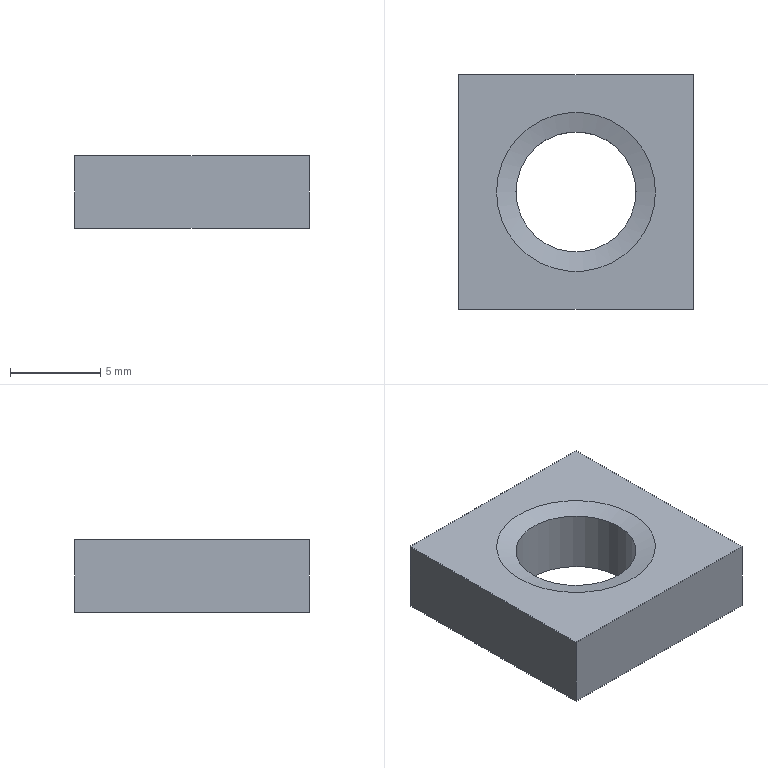Part | STEP file | Left | 1 solid | 9 faces | box 13 x 13 x 4 mm | volume 530.018 mm3 | plane 6 | cone 2 | cylinder 1 | commonest cylinder face diameters 6.647 x1
STEP:
#1=CARTESIAN_POINT('',(0.,0.,0.));
#2=DIRECTION('',(0.,0.,1.));
#3=DIRECTION('',(1.,0.,0.));
#4=AXIS2_PLACEMENT_3D('',#1,#2,#3);
#5=CARTESIAN_POINT('',(-6.5,-6.5,0.));
#6=VERTEX_POINT('',#5);
#7=CARTESIAN_POINT('',(-6.5,-6.5,4.));
#8=VERTEX_POINT('',#7);
#9=CARTESIAN_POINT('',(-6.5,-6.5,0.));
#10=DIRECTION('',(0.,0.,1.));
#11=VECTOR('',#10,1.);
#12=LINE('',#9,#11);
#13=CARTESIAN_POINT('',(-6.5,-6.5,0.));
#14=DIRECTION('',(1.,0.,0.));
#15=DIRECTION('',(0.,0.,1.));
#16=AXIS2_PLACEMENT_3D('',#13,#14,#15);
#17=PLANE('',#16);
#18=CARTESIAN_POINT('',(0.,0.));
#19=DIRECTION('',(1.,0.));
#20=VECTOR('',#19,1.);
#21=LINE('',#18,#20);
#22=(GEOMETRIC_REPRESENTATION_CONTEXT(2)PARAMETRIC_REPRESENTATION_CONTEXT()REPRESENTATION_CONTEXT('',''));
#23=DEFINITIONAL_REPRESENTATION('',(#21),#22);
#24=PCURVE('',#17,#23);
#25=CARTESIAN_POINT('',(-6.5,-6.5,0.));
#26=DIRECTION('',(0.,1.,0.));
#27=DIRECTION('',(0.,0.,1.));
#28=AXIS2_PLACEMENT_3D('',#25,#26,#27);
#29=PLANE('',#28);
#30=CARTESIAN_POINT('',(0.,0.));
#31=DIRECTION('',(1.,0.));
#32=VECTOR('',#31,1.);
#33=LINE('',#30,#32);
#34=(GEOMETRIC_REPRESENTATION_CONTEXT(2)PARAMETRIC_REPRESENTATION_CONTEXT()REPRESENTATION_CONTEXT('',''));
#35=DEFINITIONAL_REPRESENTATION('',(#33),#34);
#36=PCURVE('',#29,#35);
#37=SURFACE_CURVE('',#12,(#24,#36),.PCURVE_S1.);
#38=EDGE_CURVE('',#6,#8,#37,.T.);
#39=ORIENTED_EDGE('',*,*,#38,.F.);
#40=CARTESIAN_POINT('',(-6.5,6.5,0.));
#41=VERTEX_POINT('',#40);
#42=CARTESIAN_POINT('',(-6.5,-6.5,0.));
#43=DIRECTION('',(0.,1.,0.));
#44=VECTOR('',#43,1.);
#45=LINE('',#42,#44);
#46=CARTESIAN_POINT('',(0.,0.));
#47=DIRECTION('',(0.,-1.));
#48=VECTOR('',#47,1.);
#49=LINE('',#46,#48);
#50=(GEOMETRIC_REPRESENTATION_CONTEXT(2)PARAMETRIC_REPRESENTATION_CONTEXT()REPRESENTATION_CONTEXT('',''));
#51=DEFINITIONAL_REPRESENTATION('',(#49),#50);
#52=PCURVE('',#17,#51);
#53=CARTESIAN_POINT('',(-6.5,-6.5,0.));
#54=DIRECTION('',(0.,0.,1.));
#55=DIRECTION('',(1.,0.,0.));
#56=AXIS2_PLACEMENT_3D('',#53,#54,#55);
#57=PLANE('',#56);
#58=CARTESIAN_POINT('',(0.,0.));
#59=DIRECTION('',(0.,1.));
#60=VECTOR('',#59,1.);
#61=LINE('',#58,#60);
#62=(GEOMETRIC_REPRESENTATION_CONTEXT(2)PARAMETRIC_REPRESENTATION_CONTEXT()REPRESENTATION_CONTEXT('',''));
#63=DEFINITIONAL_REPRESENTATION('',(#61),#62);
#64=PCURVE('',#57,#63);
#65=SURFACE_CURVE('',#45,(#52,#64),.PCURVE_S1.);
#66=EDGE_CURVE('',#6,#41,#65,.T.);
#67=ORIENTED_EDGE('',*,*,#66,.T.);
#68=CARTESIAN_POINT('',(-6.5,6.5,4.));
#69=VERTEX_POINT('',#68);
#70=CARTESIAN_POINT('',(-6.5,6.5,0.));
#71=DIRECTION('',(0.,0.,1.));
#72=VECTOR('',#71,1.);
#73=LINE('',#70,#72);
#74=CARTESIAN_POINT('',(0.,-13.));
#75=DIRECTION('',(1.,0.));
#76=VECTOR('',#75,1.);
#77=LINE('',#74,#76);
#78=(GEOMETRIC_REPRESENTATION_CONTEXT(2)PARAMETRIC_REPRESENTATION_CONTEXT()REPRESENTATION_CONTEXT('',''));
#79=DEFINITIONAL_REPRESENTATION('',(#77),#78);
#80=PCURVE('',#17,#79);
#81=CARTESIAN_POINT('',(-6.5,6.5,0.));
#82=DIRECTION('',(0.,1.,0.));
#83=DIRECTION('',(0.,0.,1.));
#84=AXIS2_PLACEMENT_3D('',#81,#82,#83);
#85=PLANE('',#84);
#86=CARTESIAN_POINT('',(0.,0.));
#87=DIRECTION('',(1.,0.));
#88=VECTOR('',#87,1.);
#89=LINE('',#86,#88);
#90=(GEOMETRIC_REPRESENTATION_CONTEXT(2)PARAMETRIC_REPRESENTATION_CONTEXT()REPRESENTATION_CONTEXT('',''));
#91=DEFINITIONAL_REPRESENTATION('',(#89),#90);
#92=PCURVE('',#85,#91);
#93=SURFACE_CURVE('',#73,(#80,#92),.PCURVE_S1.);
#94=EDGE_CURVE('',#41,#69,#93,.T.);
#95=ORIENTED_EDGE('',*,*,#94,.T.);
#96=CARTESIAN_POINT('',(-6.5,-6.5,4.));
#97=DIRECTION('',(0.,1.,0.));
#98=VECTOR('',#97,1.);
#99=LINE('',#96,#98);
#100=CARTESIAN_POINT('',(4.,0.));
#101=DIRECTION('',(0.,-1.));
#102=VECTOR('',#101,1.);
#103=LINE('',#100,#102);
#104=(GEOMETRIC_REPRESENTATION_CONTEXT(2)PARAMETRIC_REPRESENTATION_CONTEXT()REPRESENTATION_CONTEXT('',''));
#105=DEFINITIONAL_REPRESENTATION('',(#103),#104);
#106=PCURVE('',#17,#105);
#107=CARTESIAN_POINT('',(-6.5,-6.5,4.));
#108=DIRECTION('',(0.,0.,1.));
#109=DIRECTION('',(1.,0.,0.));
#110=AXIS2_PLACEMENT_3D('',#107,#108,#109);
#111=PLANE('',#110);
#112=CARTESIAN_POINT('',(0.,0.));
#113=DIRECTION('',(0.,1.));
#114=VECTOR('',#113,1.);
#115=LINE('',#112,#114);
#116=(GEOMETRIC_REPRESENTATION_CONTEXT(2)PARAMETRIC_REPRESENTATION_CONTEXT()REPRESENTATION_CONTEXT('',''));
#117=DEFINITIONAL_REPRESENTATION('',(#115),#116);
#118=PCURVE('',#111,#117);
#119=SURFACE_CURVE('',#99,(#106,#118),.PCURVE_S1.);
#120=EDGE_CURVE('',#8,#69,#119,.T.);
#121=ORIENTED_EDGE('',*,*,#120,.F.);
#122=EDGE_LOOP('',(#39,#67,#95,#121));
#123=FACE_BOUND('',#122,.F.);
#124=ADVANCED_FACE('',(#123),#17,.F.);
#125=CARTESIAN_POINT('',(6.5,-6.5,0.));
#126=VERTEX_POINT('',#125);
#127=CARTESIAN_POINT('',(-6.5,-6.5,0.));
#128=DIRECTION('',(1.,0.,0.));
#129=VECTOR('',#128,1.);
#130=LINE('',#127,#129);
#131=CARTESIAN_POINT('',(0.,0.));
#132=DIRECTION('',(0.,1.));
#133=VECTOR('',#132,1.);
#134=LINE('',#131,#133);
#135=(GEOMETRIC_REPRESENTATION_CONTEXT(2)PARAMETRIC_REPRESENTATION_CONTEXT()REPRESENTATION_CONTEXT('',''));
#136=DEFINITIONAL_REPRESENTATION('',(#134),#135);
#137=PCURVE('',#29,#136);
#138=CARTESIAN_POINT('',(0.,0.));
#139=DIRECTION('',(1.,0.));
#140=VECTOR('',#139,1.);
#141=LINE('',#138,#140);
#142=(GEOMETRIC_REPRESENTATION_CONTEXT(2)PARAMETRIC_REPRESENTATION_CONTEXT()REPRESENTATION_CONTEXT('',''));
#143=DEFINITIONAL_REPRESENTATION('',(#141),#142);
#144=PCURVE('',#57,#143);
#145=SURFACE_CURVE('',#130,(#137,#144),.PCURVE_S1.);
#146=EDGE_CURVE('',#6,#126,#145,.T.);
#147=ORIENTED_EDGE('',*,*,#146,.F.);
#148=ORIENTED_EDGE('',*,*,#38,.T.);
#149=CARTESIAN_POINT('',(6.5,-6.5,4.));
#150=VERTEX_POINT('',#149);
#151=CARTESIAN_POINT('',(-6.5,-6.5,4.));
#152=DIRECTION('',(1.,0.,0.));
#153=VECTOR('',#152,1.);
#154=LINE('',#151,#153);
#155=CARTESIAN_POINT('',(4.,0.));
#156=DIRECTION('',(0.,1.));
#157=VECTOR('',#156,1.);
#158=LINE('',#155,#157);
#159=(GEOMETRIC_REPRESENTATION_CONTEXT(2)PARAMETRIC_REPRESENTATION_CONTEXT()REPRESENTATION_CONTEXT('',''));
#160=DEFINITIONAL_REPRESENTATION('',(#158),#159);
#161=PCURVE('',#29,#160);
#162=CARTESIAN_POINT('',(0.,0.));
#163=DIRECTION('',(1.,0.));
#164=VECTOR('',#163,1.);
#165=LINE('',#162,#164);
#166=(GEOMETRIC_REPRESENTATION_CONTEXT(2)PARAMETRIC_REPRESENTATION_CONTEXT()REPRESENTATION_CONTEXT('',''));
#167=DEFINITIONAL_REPRESENTATION('',(#165),#166);
#168=PCURVE('',#111,#167);
#169=SURFACE_CURVE('',#154,(#161,#168),.PCURVE_S1.);
#170=EDGE_CURVE('',#8,#150,#169,.T.);
#171=ORIENTED_EDGE('',*,*,#170,.T.);
#172=CARTESIAN_POINT('',(6.5,-6.5,0.));
#173=DIRECTION('',(0.,0.,1.));
#174=VECTOR('',#173,1.);
#175=LINE('',#172,#174);
#176=CARTESIAN_POINT('',(0.,13.));
#177=DIRECTION('',(1.,0.));
#178=VECTOR('',#177,1.);
#179=LINE('',#176,#178);
#180=(GEOMETRIC_REPRESENTATION_CONTEXT(2)PARAMETRIC_REPRESENTATION_CONTEXT()REPRESENTATION_CONTEXT('',''));
#181=DEFINITIONAL_REPRESENTATION('',(#179),#180);
#182=PCURVE('',#29,#181);
#183=CARTESIAN_POINT('',(6.5,-6.5,0.));
#184=DIRECTION('',(1.,0.,0.));
#185=DIRECTION('',(0.,0.,1.));
#186=AXIS2_PLACEMENT_3D('',#183,#184,#185);
#187=PLANE('',#186);
#188=CARTESIAN_POINT('',(0.,0.));
#189=DIRECTION('',(1.,0.));
#190=VECTOR('',#189,1.);
#191=LINE('',#188,#190);
#192=(GEOMETRIC_REPRESENTATION_CONTEXT(2)PARAMETRIC_REPRESENTATION_CONTEXT()REPRESENTATION_CONTEXT('',''));
#193=DEFINITIONAL_REPRESENTATION('',(#191),#192);
#194=PCURVE('',#187,#193);
#195=SURFACE_CURVE('',#175,(#182,#194),.PCURVE_S1.);
#196=EDGE_CURVE('',#126,#150,#195,.T.);
#197=ORIENTED_EDGE('',*,*,#196,.F.);
#198=EDGE_LOOP('',(#147,#148,#171,#197));
#199=FACE_BOUND('',#198,.F.);
#200=ADVANCED_FACE('',(#199),#29,.F.);
#201=ORIENTED_EDGE('',*,*,#120,.F.);
#202=ORIENTED_EDGE('',*,*,#170,.T.);
#203=CARTESIAN_POINT('',(6.5,6.5,4.));
#204=VERTEX_POINT('',#203);
#205=CARTESIAN_POINT('',(6.5,-6.5,4.));
#206=DIRECTION('',(0.,1.,0.));
#207=VECTOR('',#206,1.);
#208=LINE('',#205,#207);
#209=CARTESIAN_POINT('',(13.,0.));
#210=DIRECTION('',(0.,1.));
#211=VECTOR('',#210,1.);
#212=LINE('',#209,#211);
#213=(GEOMETRIC_REPRESENTATION_CONTEXT(2)PARAMETRIC_REPRESENTATION_CONTEXT()REPRESENTATION_CONTEXT('',''));
#214=DEFINITIONAL_REPRESENTATION('',(#212),#213);
#215=PCURVE('',#111,#214);
#216=CARTESIAN_POINT('',(4.,0.));
#217=DIRECTION('',(0.,-1.));
#218=VECTOR('',#217,1.);
#219=LINE('',#216,#218);
#220=(GEOMETRIC_REPRESENTATION_CONTEXT(2)PARAMETRIC_REPRESENTATION_CONTEXT()REPRESENTATION_CONTEXT('',''));
#221=DEFINITIONAL_REPRESENTATION('',(#219),#220);
#222=PCURVE('',#187,#221);
#223=SURFACE_CURVE('',#208,(#215,#222),.PCURVE_S1.);
#224=EDGE_CURVE('',#150,#204,#223,.T.);
#225=ORIENTED_EDGE('',*,*,#224,.T.);
#226=CARTESIAN_POINT('',(-6.5,6.5,4.));
#227=DIRECTION('',(1.,0.,0.));
#228=VECTOR('',#227,1.);
#229=LINE('',#226,#228);
#230=CARTESIAN_POINT('',(0.,13.));
#231=DIRECTION('',(1.,0.));
#232=VECTOR('',#231,1.);
#233=LINE('',#230,#232);
#234=(GEOMETRIC_REPRESENTATION_CONTEXT(2)PARAMETRIC_REPRESENTATION_CONTEXT()REPRESENTATION_CONTEXT('',''));
#235=DEFINITIONAL_REPRESENTATION('',(#233),#234);
#236=PCURVE('',#111,#235);
#237=CARTESIAN_POINT('',(4.,0.));
#238=DIRECTION('',(0.,1.));
#239=VECTOR('',#238,1.);
#240=LINE('',#237,#239);
#241=(GEOMETRIC_REPRESENTATION_CONTEXT(2)PARAMETRIC_REPRESENTATION_CONTEXT()REPRESENTATION_CONTEXT('',''));
#242=DEFINITIONAL_REPRESENTATION('',(#240),#241);
#243=PCURVE('',#85,#242);
#244=SURFACE_CURVE('',#229,(#236,#243),.PCURVE_S1.);
#245=EDGE_CURVE('',#69,#204,#244,.T.);
#246=ORIENTED_EDGE('',*,*,#245,.F.);
#247=EDGE_LOOP('',(#201,#202,#225,#246));
#248=FACE_BOUND('',#247,.T.);
#249=CARTESIAN_POINT('',(4.4,0.,4.));
#250=VERTEX_POINT('',#249);
#251=CARTESIAN_POINT('',(0.,0.,4.));
#252=DIRECTION('',(0.,0.,1.));
#253=DIRECTION('',(1.,0.,0.));
#254=AXIS2_PLACEMENT_3D('',#251,#252,#253);
#255=CIRCLE('',#254,4.4);
#256=CARTESIAN_POINT('',(6.5,6.5));
#257=DIRECTION('',(1.,0.));
#258=AXIS2_PLACEMENT_2D('',#256,#257);
#259=CIRCLE('',#258,4.4);
#260=(GEOMETRIC_REPRESENTATION_CONTEXT(2)PARAMETRIC_REPRESENTATION_CONTEXT()REPRESENTATION_CONTEXT('',''));
#261=DEFINITIONAL_REPRESENTATION('',(#259),#260);
#262=PCURVE('',#111,#261);
#263=CARTESIAN_POINT('',(0.,0.,3.712));
#264=DIRECTION('',(0.,0.,1.));
#265=DIRECTION('',(1.,0.,0.));
#266=AXIS2_PLACEMENT_3D('',#263,#264,#265);
#267=CONICAL_SURFACE('',#266,3.323,1.309);
#268=CARTESIAN_POINT('',(0.,0.2885));
#269=DIRECTION('',(1.,0.));
#270=VECTOR('',#269,1.);
#271=LINE('',#268,#270);
#272=(GEOMETRIC_REPRESENTATION_CONTEXT(2)PARAMETRIC_REPRESENTATION_CONTEXT()REPRESENTATION_CONTEXT('',''));
#273=DEFINITIONAL_REPRESENTATION('',(#271),#272);
#274=PCURVE('',#267,#273);
#275=SURFACE_CURVE('',#255,(#262,#274),.PCURVE_S1.);
#276=EDGE_CURVE('',#250,#250,#275,.T.);
#277=ORIENTED_EDGE('',*,*,#276,.F.);
#278=EDGE_LOOP('',(#277));
#279=FACE_BOUND('',#278,.T.);
#280=ADVANCED_FACE('',(#248,#279),#111,.T.);
#281=CARTESIAN_POINT('',(6.5,6.5,0.));
#282=VERTEX_POINT('',#281);
#283=CARTESIAN_POINT('',(-6.5,6.5,0.));
#284=DIRECTION('',(1.,0.,0.));
#285=VECTOR('',#284,1.);
#286=LINE('',#283,#285);
#287=CARTESIAN_POINT('',(0.,0.));
#288=DIRECTION('',(0.,1.));
#289=VECTOR('',#288,1.);
#290=LINE('',#287,#289);
#291=(GEOMETRIC_REPRESENTATION_CONTEXT(2)PARAMETRIC_REPRESENTATION_CONTEXT()REPRESENTATION_CONTEXT('',''));
#292=DEFINITIONAL_REPRESENTATION('',(#290),#291);
#293=PCURVE('',#85,#292);
#294=CARTESIAN_POINT('',(0.,13.));
#295=DIRECTION('',(1.,0.));
#296=VECTOR('',#295,1.);
#297=LINE('',#294,#296);
#298=(GEOMETRIC_REPRESENTATION_CONTEXT(2)PARAMETRIC_REPRESENTATION_CONTEXT()REPRESENTATION_CONTEXT('',''));
#299=DEFINITIONAL_REPRESENTATION('',(#297),#298);
#300=PCURVE('',#57,#299);
#301=SURFACE_CURVE('',#286,(#293,#300),.PCURVE_S1.);
#302=EDGE_CURVE('',#41,#282,#301,.T.);
#303=ORIENTED_EDGE('',*,*,#302,.F.);
#304=ORIENTED_EDGE('',*,*,#94,.T.);
#305=ORIENTED_EDGE('',*,*,#245,.T.);
#306=CARTESIAN_POINT('',(6.5,6.5,0.));
#307=DIRECTION('',(0.,0.,1.));
#308=VECTOR('',#307,1.);
#309=LINE('',#306,#308);
#310=CARTESIAN_POINT('',(0.,13.));
#311=DIRECTION('',(1.,0.));
#312=VECTOR('',#311,1.);
#313=LINE('',#310,#312);
#314=(GEOMETRIC_REPRESENTATION_CONTEXT(2)PARAMETRIC_REPRESENTATION_CONTEXT()REPRESENTATION_CONTEXT('',''));
#315=DEFINITIONAL_REPRESENTATION('',(#313),#314);
#316=PCURVE('',#85,#315);
#317=CARTESIAN_POINT('',(0.,-13.));
#318=DIRECTION('',(1.,0.));
#319=VECTOR('',#318,1.);
#320=LINE('',#317,#319);
#321=(GEOMETRIC_REPRESENTATION_CONTEXT(2)PARAMETRIC_REPRESENTATION_CONTEXT()REPRESENTATION_CONTEXT('',''));
#322=DEFINITIONAL_REPRESENTATION('',(#320),#321);
#323=PCURVE('',#187,#322);
#324=SURFACE_CURVE('',#309,(#316,#323),.PCURVE_S1.);
#325=EDGE_CURVE('',#282,#204,#324,.T.);
#326=ORIENTED_EDGE('',*,*,#325,.F.);
#327=EDGE_LOOP('',(#303,#304,#305,#326));
#328=FACE_BOUND('',#327,.T.);
#329=ADVANCED_FACE('',(#328),#85,.T.);
#330=ORIENTED_EDGE('',*,*,#66,.F.);
#331=ORIENTED_EDGE('',*,*,#146,.T.);
#332=CARTESIAN_POINT('',(6.5,-6.5,0.));
#333=DIRECTION('',(0.,1.,0.));
#334=VECTOR('',#333,1.);
#335=LINE('',#332,#334);
#336=CARTESIAN_POINT('',(13.,0.));
#337=DIRECTION('',(0.,1.));
#338=VECTOR('',#337,1.);
#339=LINE('',#336,#338);
#340=(GEOMETRIC_REPRESENTATION_CONTEXT(2)PARAMETRIC_REPRESENTATION_CONTEXT()REPRESENTATION_CONTEXT('',''));
#341=DEFINITIONAL_REPRESENTATION('',(#339),#340);
#342=PCURVE('',#57,#341);
#343=CARTESIAN_POINT('',(0.,0.));
#344=DIRECTION('',(0.,-1.));
#345=VECTOR('',#344,1.);
#346=LINE('',#343,#345);
#347=(GEOMETRIC_REPRESENTATION_CONTEXT(2)PARAMETRIC_REPRESENTATION_CONTEXT()REPRESENTATION_CONTEXT('',''));
#348=DEFINITIONAL_REPRESENTATION('',(#346),#347);
#349=PCURVE('',#187,#348);
#350=SURFACE_CURVE('',#335,(#342,#349),.PCURVE_S1.);
#351=EDGE_CURVE('',#126,#282,#350,.T.);
#352=ORIENTED_EDGE('',*,*,#351,.T.);
#353=ORIENTED_EDGE('',*,*,#302,.F.);
#354=EDGE_LOOP('',(#330,#331,#352,#353));
#355=FACE_BOUND('',#354,.F.);
#356=CARTESIAN_POINT('',(4.4,0.,0.));
#357=VERTEX_POINT('',#356);
#358=CARTESIAN_POINT('',(0.,0.,0.));
#359=DIRECTION('',(0.,0.,1.));
#360=DIRECTION('',(1.,0.,0.));
#361=AXIS2_PLACEMENT_3D('',#358,#359,#360);
#362=CIRCLE('',#361,4.4);
#363=CARTESIAN_POINT('',(6.5,6.5));
#364=DIRECTION('',(1.,0.));
#365=AXIS2_PLACEMENT_2D('',#363,#364);
#366=CIRCLE('',#365,4.4);
#367=(GEOMETRIC_REPRESENTATION_CONTEXT(2)PARAMETRIC_REPRESENTATION_CONTEXT()REPRESENTATION_CONTEXT('',''));
#368=DEFINITIONAL_REPRESENTATION('',(#366),#367);
#369=PCURVE('',#57,#368);
#370=CARTESIAN_POINT('',(0.,0.,0.));
#371=DIRECTION('',(0.,0.,-1.));
#372=DIRECTION('',(1.,0.,0.));
#373=AXIS2_PLACEMENT_3D('',#370,#371,#372);
#374=CONICAL_SURFACE('',#373,4.4,1.309);
#375=CARTESIAN_POINT('',(6.283,0.));
#376=DIRECTION('',(-1.,0.));
#377=VECTOR('',#376,1.);
#378=LINE('',#375,#377);
#379=(GEOMETRIC_REPRESENTATION_CONTEXT(2)PARAMETRIC_REPRESENTATION_CONTEXT()REPRESENTATION_CONTEXT('',''));
#380=DEFINITIONAL_REPRESENTATION('',(#378),#379);
#381=PCURVE('',#374,#380);
#382=SURFACE_CURVE('',#362,(#369,#381),.PCURVE_S1.);
#383=EDGE_CURVE('',#357,#357,#382,.T.);
#384=ORIENTED_EDGE('',*,*,#383,.F.);
#385=EDGE_LOOP('',(#384));
#386=FACE_BOUND('',#385,.F.);
#387=ADVANCED_FACE('',(#355,#386),#57,.F.);
#388=ORIENTED_EDGE('',*,*,#196,.F.);
#389=ORIENTED_EDGE('',*,*,#351,.T.);
#390=ORIENTED_EDGE('',*,*,#325,.T.);
#391=ORIENTED_EDGE('',*,*,#224,.F.);
#392=EDGE_LOOP('',(#388,#389,#390,#391));
#393=FACE_BOUND('',#392,.T.);
#394=ADVANCED_FACE('',(#393),#187,.T.);
#395=CARTESIAN_POINT('',(3.323,0.,3.712));
#396=VERTEX_POINT('',#395);
#397=CARTESIAN_POINT('',(3.323,0.,3.712));
#398=DIRECTION('',(0.9659,0.,0.2588));
#399=VECTOR('',#398,1.);
#400=LINE('',#397,#399);
#401=CARTESIAN_POINT('',(0.,0.));
#402=DIRECTION('',(0.,1.));
#403=VECTOR('',#402,1.);
#404=LINE('',#401,#403);
#405=(GEOMETRIC_REPRESENTATION_CONTEXT(2)PARAMETRIC_REPRESENTATION_CONTEXT()REPRESENTATION_CONTEXT('',''));
#406=DEFINITIONAL_REPRESENTATION('',(#404),#405);
#407=PCURVE('',#267,#406);
#408=CARTESIAN_POINT('',(6.283,0.));
#409=DIRECTION('',(0.,1.));
#410=VECTOR('',#409,1.);
#411=LINE('',#408,#410);
#412=(GEOMETRIC_REPRESENTATION_CONTEXT(2)PARAMETRIC_REPRESENTATION_CONTEXT()REPRESENTATION_CONTEXT('',''));
#413=DEFINITIONAL_REPRESENTATION('',(#411),#412);
#414=PCURVE('',#267,#413);
#415=SEAM_CURVE('',#400,(#407,#414),.PCURVE_S1.);
#416=EDGE_CURVE('',#396,#250,#415,.T.);
#417=ORIENTED_EDGE('',*,*,#416,.F.);
#418=CARTESIAN_POINT('',(0.,0.,3.712));
#419=DIRECTION('',(0.,0.,1.));
#420=DIRECTION('',(1.,0.,0.));
#421=AXIS2_PLACEMENT_3D('',#418,#419,#420);
#422=CIRCLE('',#421,3.323);
#423=CARTESIAN_POINT('',(0.,0.));
#424=DIRECTION('',(1.,0.));
#425=VECTOR('',#424,1.);
#426=LINE('',#423,#425);
#427=(GEOMETRIC_REPRESENTATION_CONTEXT(2)PARAMETRIC_REPRESENTATION_CONTEXT()REPRESENTATION_CONTEXT('',''));
#428=DEFINITIONAL_REPRESENTATION('',(#426),#427);
#429=PCURVE('',#267,#428);
#430=CARTESIAN_POINT('',(0.,0.,0.2885));
#431=DIRECTION('',(0.,0.,1.));
#432=DIRECTION('',(1.,0.,0.));
#433=AXIS2_PLACEMENT_3D('',#430,#431,#432);
#434=CYLINDRICAL_SURFACE('',#433,3.323);
#435=CARTESIAN_POINT('',(0.,3.423));
#436=DIRECTION('',(1.,0.));
#437=VECTOR('',#436,1.);
#438=LINE('',#435,#437);
#439=(GEOMETRIC_REPRESENTATION_CONTEXT(2)PARAMETRIC_REPRESENTATION_CONTEXT()REPRESENTATION_CONTEXT('',''));
#440=DEFINITIONAL_REPRESENTATION('',(#438),#439);
#441=PCURVE('',#434,#440);
#442=SURFACE_CURVE('',#422,(#429,#441),.PCURVE_S1.);
#443=EDGE_CURVE('',#396,#396,#442,.T.);
#444=ORIENTED_EDGE('',*,*,#443,.T.);
#445=ORIENTED_EDGE('',*,*,#416,.T.);
#446=ORIENTED_EDGE('',*,*,#276,.F.);
#447=EDGE_LOOP('',(#417,#444,#445,#446));
#448=FACE_BOUND('',#447,.F.);
#449=ADVANCED_FACE('',(#448),#267,.F.);
#450=CARTESIAN_POINT('',(3.323,0.,0.2885));
#451=VERTEX_POINT('',#450);
#452=CARTESIAN_POINT('',(4.4,0.,0.));
#453=DIRECTION('',(-0.9659,0.,0.2588));
#454=VECTOR('',#453,1.);
#455=LINE('',#452,#454);
#456=CARTESIAN_POINT('',(6.283,0.));
#457=DIRECTION('',(0.,-1.));
#458=VECTOR('',#457,1.);
#459=LINE('',#456,#458);
#460=(GEOMETRIC_REPRESENTATION_CONTEXT(2)PARAMETRIC_REPRESENTATION_CONTEXT()REPRESENTATION_CONTEXT('',''));
#461=DEFINITIONAL_REPRESENTATION('',(#459),#460);
#462=PCURVE('',#374,#461);
#463=CARTESIAN_POINT('',(0.,0.));
#464=DIRECTION('',(0.,-1.));
#465=VECTOR('',#464,1.);
#466=LINE('',#463,#465);
#467=(GEOMETRIC_REPRESENTATION_CONTEXT(2)PARAMETRIC_REPRESENTATION_CONTEXT()REPRESENTATION_CONTEXT('',''));
#468=DEFINITIONAL_REPRESENTATION('',(#466),#467);
#469=PCURVE('',#374,#468);
#470=SEAM_CURVE('',#455,(#462,#469),.PCURVE_S1.);
#471=EDGE_CURVE('',#357,#451,#470,.T.);
#472=ORIENTED_EDGE('',*,*,#471,.F.);
#473=ORIENTED_EDGE('',*,*,#383,.T.);
#474=ORIENTED_EDGE('',*,*,#471,.T.);
#475=CARTESIAN_POINT('',(0.,0.,0.2885));
#476=DIRECTION('',(0.,0.,1.));
#477=DIRECTION('',(1.,0.,0.));
#478=AXIS2_PLACEMENT_3D('',#475,#476,#477);
#479=CIRCLE('',#478,3.323);
#480=CARTESIAN_POINT('',(6.283,-0.2885));
#481=DIRECTION('',(-1.,0.));
#482=VECTOR('',#481,1.);
#483=LINE('',#480,#482);
#484=(GEOMETRIC_REPRESENTATION_CONTEXT(2)PARAMETRIC_REPRESENTATION_CONTEXT()REPRESENTATION_CONTEXT('',''));
#485=DEFINITIONAL_REPRESENTATION('',(#483),#484);
#486=PCURVE('',#374,#485);
#487=CARTESIAN_POINT('',(0.,0.));
#488=DIRECTION('',(1.,0.));
#489=VECTOR('',#488,1.);
#490=LINE('',#487,#489);
#491=(GEOMETRIC_REPRESENTATION_CONTEXT(2)PARAMETRIC_REPRESENTATION_CONTEXT()REPRESENTATION_CONTEXT('',''));
#492=DEFINITIONAL_REPRESENTATION('',(#490),#491);
#493=PCURVE('',#434,#492);
#494=SURFACE_CURVE('',#479,(#486,#493),.PCURVE_S1.);
#495=EDGE_CURVE('',#451,#451,#494,.T.);
#496=ORIENTED_EDGE('',*,*,#495,.F.);
#497=EDGE_LOOP('',(#472,#473,#474,#496));
#498=FACE_BOUND('',#497,.F.);
#499=ADVANCED_FACE('',(#498),#374,.F.);
#500=ORIENTED_EDGE('',*,*,#495,.T.);
#501=CARTESIAN_POINT('',(3.323,0.,0.2885));
#502=DIRECTION('',(0.,0.,1.));
#503=VECTOR('',#502,1.);
#504=LINE('',#501,#503);
#505=CARTESIAN_POINT('',(6.283,0.));
#506=DIRECTION('',(0.,1.));
#507=VECTOR('',#506,1.);
#508=LINE('',#505,#507);
#509=(GEOMETRIC_REPRESENTATION_CONTEXT(2)PARAMETRIC_REPRESENTATION_CONTEXT()REPRESENTATION_CONTEXT('',''));
#510=DEFINITIONAL_REPRESENTATION('',(#508),#509);
#511=PCURVE('',#434,#510);
#512=CARTESIAN_POINT('',(0.,0.));
#513=DIRECTION('',(0.,1.));
#514=VECTOR('',#513,1.);
#515=LINE('',#512,#514);
#516=(GEOMETRIC_REPRESENTATION_CONTEXT(2)PARAMETRIC_REPRESENTATION_CONTEXT()REPRESENTATION_CONTEXT('',''));
#517=DEFINITIONAL_REPRESENTATION('',(#515),#516);
#518=PCURVE('',#434,#517);
#519=SEAM_CURVE('',#504,(#511,#518),.PCURVE_S1.);
#520=EDGE_CURVE('',#451,#396,#519,.T.);
#521=ORIENTED_EDGE('',*,*,#520,.T.);
#522=ORIENTED_EDGE('',*,*,#443,.F.);
#523=ORIENTED_EDGE('',*,*,#520,.F.);
#524=EDGE_LOOP('',(#500,#521,#522,#523));
#525=FACE_BOUND('',#524,.F.);
#526=ADVANCED_FACE('',(#525),#434,.F.);
#527=CLOSED_SHELL('',(#124,#200,#280,#329,#387,#394,#449,#499,#526));
#528=MANIFOLD_SOLID_BREP('',#527);
#529=(LENGTH_UNIT()NAMED_UNIT(*)SI_UNIT(.MILLI.,.METRE.));
#530=UNCERTAINTY_MEASURE_WITH_UNIT(LENGTH_MEASURE(0.0000001),#529,'','');
#531=(NAMED_UNIT(*)PLANE_ANGLE_UNIT()SI_UNIT($,.RADIAN.));
#532=(NAMED_UNIT(*)SI_UNIT($,.STERADIAN.)SOLID_ANGLE_UNIT());
#533=(GEOMETRIC_REPRESENTATION_CONTEXT(3)GLOBAL_UNCERTAINTY_ASSIGNED_CONTEXT((#530))GLOBAL_UNIT_ASSIGNED_CONTEXT((#529,#531,#532))REPRESENTATION_CONTEXT('',''));
#534=ADVANCED_BREP_SHAPE_REPRESENTATION('',(#4,#528),#533);